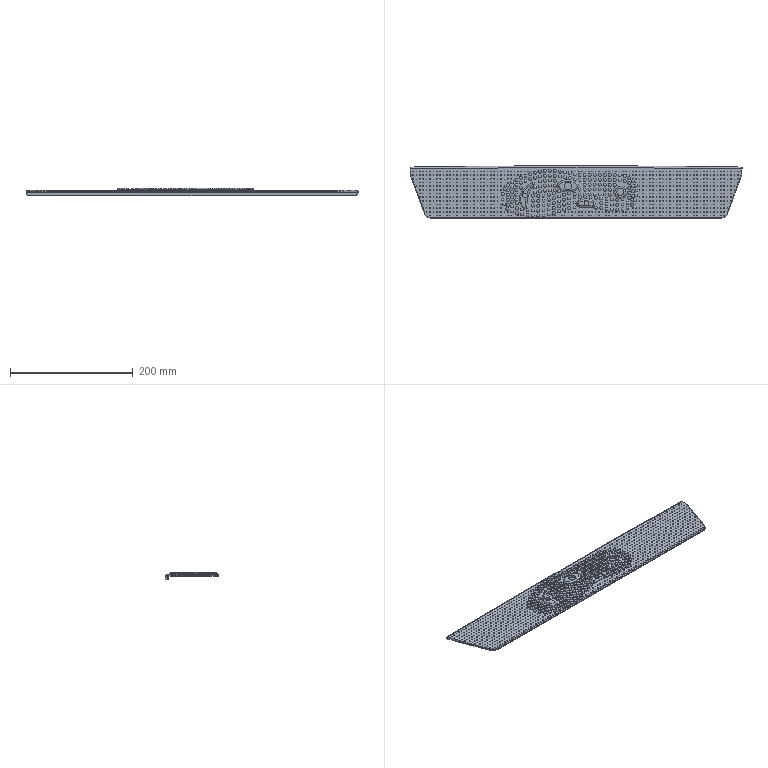Part | STEP file | ZHD 500.80R | 1 solid | 2076 faces | box 540 x 85 x 12 mm | volume 102957 mm3 | cylinder 1028 | sphere 997 | plane 26 | torus 16 | spline 9 | commonest cylinder face diameters 1 x810 4.5 x188 2 x7 8 x4 10 x2 12 x2